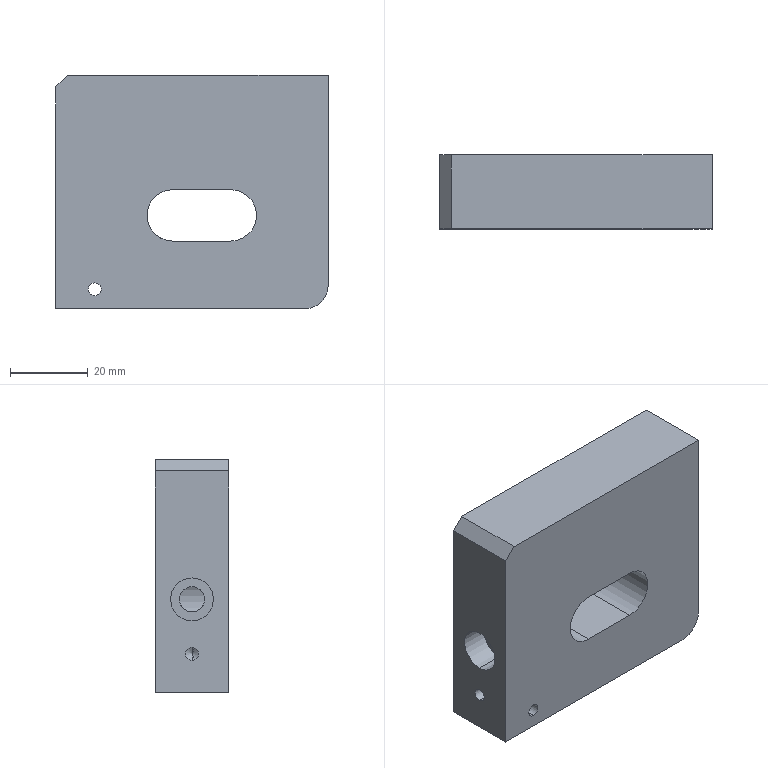Part | STEP file | adjustment limit plate | 1 solid | 31 faces | box 70 x 19 x 60 mm | volume 70894 mm3 | cylinder 15 | plane 10 | cone 6 | commonest cylinder face diameters 3.3 x4 5 x4 6.5 x2 11 x2 13.2 x2 12 x1